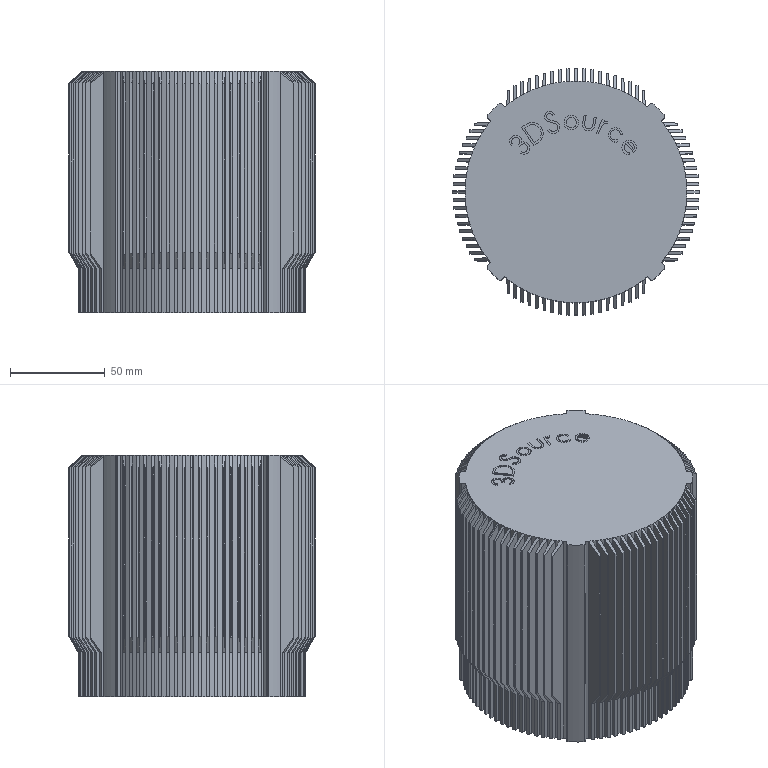Part | NX | features BREP 1 | 1 solid | 662 faces | box 130 x 130 x 127.333 mm | volume 1463982 mm3 | cylinder 302 | plane 206 | cone 154 | commonest cylinder face diameters 130 x95 117 x80 120.25 x77 2.08 x10 4.361 x8 5.406 x6